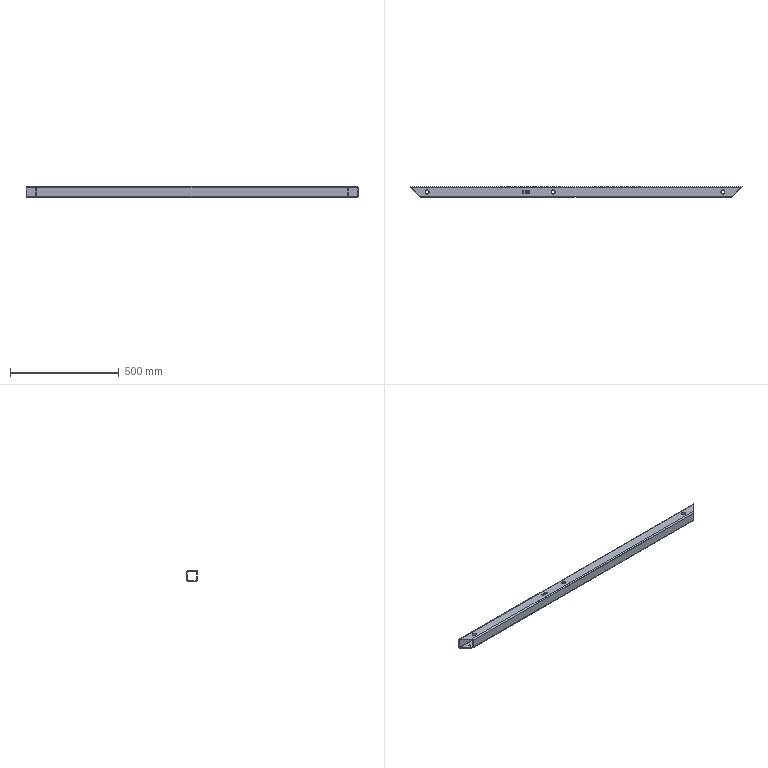Part | SolidWorks | features BaseBody 1 | 1 solid | 118 faces | box 1527 x 50 x 50 mm | volume 791850 mm3 | plane 67 | spline 30 | cylinder 21 | commonest cylinder face diameters 18 x6 18.8 x6 12 x4 6 x3 5.1 x2